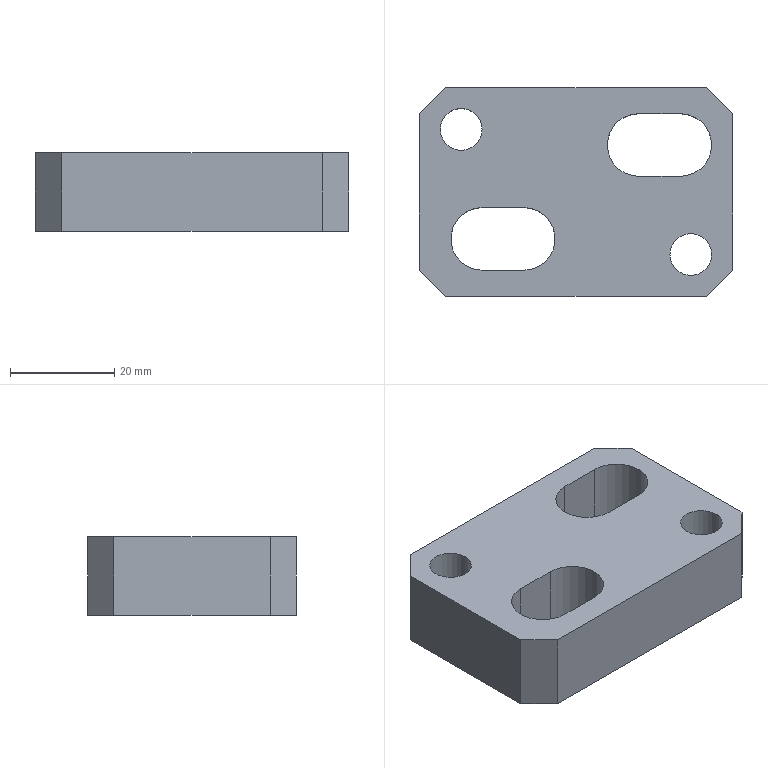Part | NX | features solid 2 | 1 solid | 20 faces | box 60 x 40 x 15 mm | volume 27469 mm3 | plane 14 | cylinder 6 | commonest cylinder face diameters 12 x4 8 x2
STEP:
#1=CARTESIAN_POINT('',(-940.,-92.5,-50.));
#2=VERTEX_POINT('',#1);
#3=CARTESIAN_POINT('',(-890.,-92.5,-50.));
#4=VERTEX_POINT('',#3);
#5=CARTESIAN_POINT('',(-945.,-92.5,-50.));
#6=DIRECTION('',(1.,0.,0.));
#7=VECTOR('',#6,1000.);
#8=LINE('',#5,#7);
#9=EDGE_CURVE('',#2,#4,#8,.T.);
#10=ORIENTED_EDGE('',*,*,#9,.T.);
#11=CARTESIAN_POINT('',(-890.,-92.5,-35.));
#12=VERTEX_POINT('',#11);
#13=CARTESIAN_POINT('',(-890.,-92.5,-35.));
#14=DIRECTION('',(0.,0.,-1.));
#15=VECTOR('',#14,1000.);
#16=LINE('',#13,#15);
#17=EDGE_CURVE('',#12,#4,#16,.T.);
#18=ORIENTED_EDGE('',*,*,#17,.F.);
#19=CARTESIAN_POINT('',(-940.,-92.5,-35.));
#20=VERTEX_POINT('',#19);
#21=CARTESIAN_POINT('',(-945.,-92.5,-35.));
#22=DIRECTION('',(1.,0.,0.));
#23=VECTOR('',#22,1000.);
#24=LINE('',#21,#23);
#25=EDGE_CURVE('',#20,#12,#24,.T.);
#26=ORIENTED_EDGE('',*,*,#25,.F.);
#27=CARTESIAN_POINT('',(-940.,-92.5,-35.));
#28=DIRECTION('',(0.,0.,-1.));
#29=VECTOR('',#28,1000.);
#30=LINE('',#27,#29);
#31=EDGE_CURVE('',#20,#2,#30,.T.);
#32=ORIENTED_EDGE('',*,*,#31,.T.);
#33=EDGE_LOOP('',(#10,#18,#26,#32));
#34=FACE_BOUND('',#33,.T.);
#35=CARTESIAN_POINT('',(-945.,-92.5,-35.));
#36=DIRECTION('',(0.,-1.,0.));
#37=DIRECTION('',(0.,0.,-1.));
#38=AXIS2_PLACEMENT_3D('',#35,#36,#37);
#39=PLANE('',#38);
#40=ADVANCED_FACE('',(#34),#39,.T.);
#41=CARTESIAN_POINT('',(-885.,-87.5,-50.));
#42=VERTEX_POINT('',#41);
#43=CARTESIAN_POINT('',(-890.,-92.5,-50.));
#44=DIRECTION('',(0.7071,0.7071,0.));
#45=VECTOR('',#44,1000.);
#46=LINE('',#43,#45);
#47=EDGE_CURVE('',#4,#42,#46,.T.);
#48=ORIENTED_EDGE('',*,*,#47,.T.);
#49=CARTESIAN_POINT('',(-885.,-87.5,-35.));
#50=VERTEX_POINT('',#49);
#51=CARTESIAN_POINT('',(-885.,-87.5,-35.));
#52=DIRECTION('',(0.,0.,-1.));
#53=VECTOR('',#52,1000.);
#54=LINE('',#51,#53);
#55=EDGE_CURVE('',#50,#42,#54,.T.);
#56=ORIENTED_EDGE('',*,*,#55,.F.);
#57=CARTESIAN_POINT('',(-890.,-92.5,-35.));
#58=DIRECTION('',(0.7071,0.7071,0.));
#59=VECTOR('',#58,1000.);
#60=LINE('',#57,#59);
#61=EDGE_CURVE('',#12,#50,#60,.T.);
#62=ORIENTED_EDGE('',*,*,#61,.F.);
#63=ORIENTED_EDGE('',*,*,#17,.T.);
#64=EDGE_LOOP('',(#48,#56,#62,#63));
#65=FACE_BOUND('',#64,.T.);
#66=CARTESIAN_POINT('',(-890.,-92.5,-35.));
#67=DIRECTION('',(0.7071,-0.7071,0.));
#68=DIRECTION('',(-0.7071,-0.7071,0.));
#69=AXIS2_PLACEMENT_3D('',#66,#67,#68);
#70=PLANE('',#69);
#71=ADVANCED_FACE('',(#65),#70,.T.);
#72=CARTESIAN_POINT('',(-885.,-57.5,-50.));
#73=VERTEX_POINT('',#72);
#74=CARTESIAN_POINT('',(-885.,-87.5,-50.));
#75=DIRECTION('',(0.,1.,0.));
#76=VECTOR('',#75,1000.);
#77=LINE('',#74,#76);
#78=EDGE_CURVE('',#42,#73,#77,.T.);
#79=ORIENTED_EDGE('',*,*,#78,.T.);
#80=CARTESIAN_POINT('',(-885.,-57.5,-35.));
#81=VERTEX_POINT('',#80);
#82=CARTESIAN_POINT('',(-885.,-57.5,-35.));
#83=DIRECTION('',(0.,0.,-1.));
#84=VECTOR('',#83,1000.);
#85=LINE('',#82,#84);
#86=EDGE_CURVE('',#81,#73,#85,.T.);
#87=ORIENTED_EDGE('',*,*,#86,.F.);
#88=CARTESIAN_POINT('',(-885.,-87.5,-35.));
#89=DIRECTION('',(0.,1.,0.));
#90=VECTOR('',#89,1000.);
#91=LINE('',#88,#90);
#92=EDGE_CURVE('',#50,#81,#91,.T.);
#93=ORIENTED_EDGE('',*,*,#92,.F.);
#94=ORIENTED_EDGE('',*,*,#55,.T.);
#95=EDGE_LOOP('',(#79,#87,#93,#94));
#96=FACE_BOUND('',#95,.T.);
#97=CARTESIAN_POINT('',(-885.,-87.5,-35.));
#98=DIRECTION('',(1.,0.,0.));
#99=DIRECTION('',(0.,-1.,0.));
#100=AXIS2_PLACEMENT_3D('',#97,#98,#99);
#101=PLANE('',#100);
#102=ADVANCED_FACE('',(#96),#101,.T.);
#103=CARTESIAN_POINT('',(-890.,-52.5,-50.));
#104=VERTEX_POINT('',#103);
#105=CARTESIAN_POINT('',(-885.,-57.5,-50.));
#106=DIRECTION('',(-0.7071,0.7071,0.));
#107=VECTOR('',#106,1000.);
#108=LINE('',#105,#107);
#109=EDGE_CURVE('',#73,#104,#108,.T.);
#110=ORIENTED_EDGE('',*,*,#109,.T.);
#111=CARTESIAN_POINT('',(-890.,-52.5,-35.));
#112=VERTEX_POINT('',#111);
#113=CARTESIAN_POINT('',(-890.,-52.5,-35.));
#114=DIRECTION('',(0.,0.,-1.));
#115=VECTOR('',#114,1000.);
#116=LINE('',#113,#115);
#117=EDGE_CURVE('',#112,#104,#116,.T.);
#118=ORIENTED_EDGE('',*,*,#117,.F.);
#119=CARTESIAN_POINT('',(-885.,-57.5,-35.));
#120=DIRECTION('',(-0.7071,0.7071,0.));
#121=VECTOR('',#120,1000.);
#122=LINE('',#119,#121);
#123=EDGE_CURVE('',#81,#112,#122,.T.);
#124=ORIENTED_EDGE('',*,*,#123,.F.);
#125=ORIENTED_EDGE('',*,*,#86,.T.);
#126=EDGE_LOOP('',(#110,#118,#124,#125));
#127=FACE_BOUND('',#126,.T.);
#128=CARTESIAN_POINT('',(-885.,-57.5,-35.));
#129=DIRECTION('',(0.7071,0.7071,0.));
#130=DIRECTION('',(0.7071,-0.7071,0.));
#131=AXIS2_PLACEMENT_3D('',#128,#129,#130);
#132=PLANE('',#131);
#133=ADVANCED_FACE('',(#127),#132,.T.);
#134=CARTESIAN_POINT('',(-940.,-52.5,-35.));
#135=VERTEX_POINT('',#134);
#136=CARTESIAN_POINT('',(-915.,-52.5,-35.));
#137=DIRECTION('',(-1.,0.,0.));
#138=VECTOR('',#137,1000.);
#139=LINE('',#136,#138);
#140=EDGE_CURVE('',#112,#135,#139,.T.);
#141=ORIENTED_EDGE('',*,*,#140,.F.);
#142=ORIENTED_EDGE('',*,*,#117,.T.);
#143=CARTESIAN_POINT('',(-940.,-52.5,-50.));
#144=VERTEX_POINT('',#143);
#145=CARTESIAN_POINT('',(-915.,-52.5,-50.));
#146=DIRECTION('',(-1.,0.,0.));
#147=VECTOR('',#146,1000.);
#148=LINE('',#145,#147);
#149=EDGE_CURVE('',#104,#144,#148,.T.);
#150=ORIENTED_EDGE('',*,*,#149,.T.);
#151=CARTESIAN_POINT('',(-940.,-52.5,-35.));
#152=DIRECTION('',(0.,0.,-1.));
#153=VECTOR('',#152,1000.);
#154=LINE('',#151,#153);
#155=EDGE_CURVE('',#135,#144,#154,.T.);
#156=ORIENTED_EDGE('',*,*,#155,.F.);
#157=EDGE_LOOP('',(#141,#142,#150,#156));
#158=FACE_BOUND('',#157,.T.);
#159=CARTESIAN_POINT('',(-915.,-52.5,-35.));
#160=DIRECTION('',(0.,1.,0.));
#161=DIRECTION('',(1.,0.,0.));
#162=AXIS2_PLACEMENT_3D('',#159,#160,#161);
#163=PLANE('',#162);
#164=ADVANCED_FACE('',(#158),#163,.T.);
#165=CARTESIAN_POINT('',(-903.,-69.5,-50.));
#166=VERTEX_POINT('',#165);
#167=CARTESIAN_POINT('',(-903.,-57.5,-50.));
#168=VERTEX_POINT('',#167);
#169=CARTESIAN_POINT('',(-903.,-63.5,-50.));
#170=DIRECTION('',(0.,0.,-1.));
#171=DIRECTION('',(-1.,0.,0.));
#172=AXIS2_PLACEMENT_3D('',#169,#170,#171);
#173=CIRCLE('',#172,6.);
#174=EDGE_CURVE('',#166,#168,#173,.T.);
#175=ORIENTED_EDGE('',*,*,#174,.T.);
#176=CARTESIAN_POINT('',(-903.,-57.5,-35.));
#177=VERTEX_POINT('',#176);
#178=CARTESIAN_POINT('',(-903.,-57.5,-35.));
#179=DIRECTION('',(0.,0.,-1.));
#180=VECTOR('',#179,1000.);
#181=LINE('',#178,#180);
#182=EDGE_CURVE('',#177,#168,#181,.T.);
#183=ORIENTED_EDGE('',*,*,#182,.F.);
#184=CARTESIAN_POINT('',(-903.,-69.5,-35.));
#185=VERTEX_POINT('',#184);
#186=CARTESIAN_POINT('',(-903.,-63.5,-35.));
#187=DIRECTION('',(0.,0.,-1.));
#188=DIRECTION('',(-1.,0.,0.));
#189=AXIS2_PLACEMENT_3D('',#186,#187,#188);
#190=CIRCLE('',#189,6.);
#191=EDGE_CURVE('',#185,#177,#190,.T.);
#192=ORIENTED_EDGE('',*,*,#191,.F.);
#193=CARTESIAN_POINT('',(-903.,-69.5,-35.));
#194=DIRECTION('',(0.,0.,-1.));
#195=VECTOR('',#194,1000.);
#196=LINE('',#193,#195);
#197=EDGE_CURVE('',#185,#166,#196,.T.);
#198=ORIENTED_EDGE('',*,*,#197,.T.);
#199=EDGE_LOOP('',(#175,#183,#192,#198));
#200=FACE_BOUND('',#199,.T.);
#201=CARTESIAN_POINT('',(-903.,-63.5,-35.));
#202=DIRECTION('',(0.,0.,-1.));
#203=DIRECTION('',(1.,0.,0.));
#204=AXIS2_PLACEMENT_3D('',#201,#202,#203);
#205=CYLINDRICAL_SURFACE('',#204,6.);
#206=ADVANCED_FACE('',(#200),#205,.F.);
#207=CARTESIAN_POINT('',(-895.,-57.5,-50.));
#208=VERTEX_POINT('',#207);
#209=CARTESIAN_POINT('',(-895.,-57.5,-50.));
#210=DIRECTION('',(-1.,0.,0.));
#211=VECTOR('',#210,1000.);
#212=LINE('',#209,#211);
#213=EDGE_CURVE('',#208,#168,#212,.T.);
#214=ORIENTED_EDGE('',*,*,#213,.F.);
#215=CARTESIAN_POINT('',(-895.,-57.5,-35.));
#216=VERTEX_POINT('',#215);
#217=CARTESIAN_POINT('',(-895.,-57.5,-35.));
#218=DIRECTION('',(0.,0.,-1.));
#219=VECTOR('',#218,1000.);
#220=LINE('',#217,#219);
#221=EDGE_CURVE('',#216,#208,#220,.T.);
#222=ORIENTED_EDGE('',*,*,#221,.F.);
#223=CARTESIAN_POINT('',(-895.,-57.5,-35.));
#224=DIRECTION('',(-1.,0.,0.));
#225=VECTOR('',#224,1000.);
#226=LINE('',#223,#225);
#227=EDGE_CURVE('',#216,#177,#226,.T.);
#228=ORIENTED_EDGE('',*,*,#227,.T.);
#229=ORIENTED_EDGE('',*,*,#182,.T.);
#230=EDGE_LOOP('',(#214,#222,#228,#229));
#231=FACE_BOUND('',#230,.T.);
#232=CARTESIAN_POINT('',(-895.,-57.5,-35.));
#233=DIRECTION('',(0.,1.,0.));
#234=DIRECTION('',(0.,0.,1.));
#235=AXIS2_PLACEMENT_3D('',#232,#233,#234);
#236=PLANE('',#235);
#237=ADVANCED_FACE('',(#231),#236,.F.);
#238=CARTESIAN_POINT('',(-895.,-69.5,-50.));
#239=VERTEX_POINT('',#238);
#240=CARTESIAN_POINT('',(-895.,-63.5,-50.));
#241=DIRECTION('',(0.,0.,-1.));
#242=DIRECTION('',(-1.,0.,0.));
#243=AXIS2_PLACEMENT_3D('',#240,#241,#242);
#244=CIRCLE('',#243,6.);
#245=EDGE_CURVE('',#208,#239,#244,.T.);
#246=ORIENTED_EDGE('',*,*,#245,.T.);
#247=CARTESIAN_POINT('',(-895.,-69.5,-35.));
#248=VERTEX_POINT('',#247);
#249=CARTESIAN_POINT('',(-895.,-69.5,-35.));
#250=DIRECTION('',(0.,0.,-1.));
#251=VECTOR('',#250,1000.);
#252=LINE('',#249,#251);
#253=EDGE_CURVE('',#248,#239,#252,.T.);
#254=ORIENTED_EDGE('',*,*,#253,.F.);
#255=CARTESIAN_POINT('',(-895.,-63.5,-35.));
#256=DIRECTION('',(0.,0.,-1.));
#257=DIRECTION('',(-1.,0.,0.));
#258=AXIS2_PLACEMENT_3D('',#255,#256,#257);
#259=CIRCLE('',#258,6.);
#260=EDGE_CURVE('',#216,#248,#259,.T.);
#261=ORIENTED_EDGE('',*,*,#260,.F.);
#262=ORIENTED_EDGE('',*,*,#221,.T.);
#263=EDGE_LOOP('',(#246,#254,#261,#262));
#264=FACE_BOUND('',#263,.T.);
#265=CARTESIAN_POINT('',(-895.,-63.5,-35.));
#266=DIRECTION('',(0.,0.,-1.));
#267=DIRECTION('',(1.,0.,0.));
#268=AXIS2_PLACEMENT_3D('',#265,#266,#267);
#269=CYLINDRICAL_SURFACE('',#268,6.);
#270=ADVANCED_FACE('',(#264),#269,.F.);
#271=CARTESIAN_POINT('',(-903.,-69.5,-35.));
#272=DIRECTION('',(1.,0.,0.));
#273=VECTOR('',#272,1000.);
#274=LINE('',#271,#273);
#275=EDGE_CURVE('',#185,#248,#274,.T.);
#276=ORIENTED_EDGE('',*,*,#275,.T.);
#277=ORIENTED_EDGE('',*,*,#253,.T.);
#278=CARTESIAN_POINT('',(-903.,-69.5,-50.));
#279=DIRECTION('',(1.,0.,0.));
#280=VECTOR('',#279,1000.);
#281=LINE('',#278,#280);
#282=EDGE_CURVE('',#166,#239,#281,.T.);
#283=ORIENTED_EDGE('',*,*,#282,.F.);
#284=ORIENTED_EDGE('',*,*,#197,.F.);
#285=EDGE_LOOP('',(#276,#277,#283,#284));
#286=FACE_BOUND('',#285,.T.);
#287=CARTESIAN_POINT('',(-903.,-69.5,-35.));
#288=DIRECTION('',(0.,-1.,0.));
#289=DIRECTION('',(-1.,0.,0.));
#290=AXIS2_PLACEMENT_3D('',#287,#288,#289);
#291=PLANE('',#290);
#292=ADVANCED_FACE('',(#286),#291,.F.);
#293=CARTESIAN_POINT('',(-941.,-60.5,-35.));
#294=VERTEX_POINT('',#293);
#295=CARTESIAN_POINT('',(-937.,-60.5,-35.));
#296=DIRECTION('',(0.,0.,-1.));
#297=DIRECTION('',(-1.,0.,0.));
#298=AXIS2_PLACEMENT_3D('',#295,#296,#297);
#299=CIRCLE('',#298,4.);
#300=EDGE_CURVE('',#294,#294,#299,.T.);
#301=ORIENTED_EDGE('',*,*,#300,.F.);
#302=EDGE_LOOP('',(#301));
#303=FACE_BOUND('',#302,.T.);
#304=CARTESIAN_POINT('',(-941.,-60.5,-50.));
#305=VERTEX_POINT('',#304);
#306=CARTESIAN_POINT('',(-937.,-60.5,-50.));
#307=DIRECTION('',(0.,0.,-1.));
#308=DIRECTION('',(-1.,0.,0.));
#309=AXIS2_PLACEMENT_3D('',#306,#307,#308);
#310=CIRCLE('',#309,4.);
#311=EDGE_CURVE('',#305,#305,#310,.T.);
#312=ORIENTED_EDGE('',*,*,#311,.T.);
#313=EDGE_LOOP('',(#312));
#314=FACE_BOUND('',#313,.T.);
#315=CARTESIAN_POINT('',(-937.,-60.5,-35.));
#316=DIRECTION('',(0.,0.,-1.));
#317=DIRECTION('',(1.,0.,0.));
#318=AXIS2_PLACEMENT_3D('',#315,#316,#317);
#319=CYLINDRICAL_SURFACE('',#318,4.);
#320=ADVANCED_FACE('',(#303,#314),#319,.F.);
#321=CARTESIAN_POINT('',(-933.,-87.5,-50.));
#322=VERTEX_POINT('',#321);
#323=CARTESIAN_POINT('',(-933.,-75.5,-50.));
#324=VERTEX_POINT('',#323);
#325=CARTESIAN_POINT('',(-933.,-81.5,-50.));
#326=DIRECTION('',(0.,0.,-1.));
#327=DIRECTION('',(-1.,0.,0.));
#328=AXIS2_PLACEMENT_3D('',#325,#326,#327);
#329=CIRCLE('',#328,6.);
#330=EDGE_CURVE('',#322,#324,#329,.T.);
#331=ORIENTED_EDGE('',*,*,#330,.T.);
#332=CARTESIAN_POINT('',(-933.,-75.5,-35.));
#333=VERTEX_POINT('',#332);
#334=CARTESIAN_POINT('',(-933.,-75.5,-35.));
#335=DIRECTION('',(0.,0.,-1.));
#336=VECTOR('',#335,1000.);
#337=LINE('',#334,#336);
#338=EDGE_CURVE('',#333,#324,#337,.T.);
#339=ORIENTED_EDGE('',*,*,#338,.F.);
#340=CARTESIAN_POINT('',(-933.,-87.5,-35.));
#341=VERTEX_POINT('',#340);
#342=CARTESIAN_POINT('',(-933.,-81.5,-35.));
#343=DIRECTION('',(0.,0.,-1.));
#344=DIRECTION('',(-1.,0.,0.));
#345=AXIS2_PLACEMENT_3D('',#342,#343,#344);
#346=CIRCLE('',#345,6.);
#347=EDGE_CURVE('',#341,#333,#346,.T.);
#348=ORIENTED_EDGE('',*,*,#347,.F.);
#349=CARTESIAN_POINT('',(-933.,-87.5,-35.));
#350=DIRECTION('',(0.,0.,-1.));
#351=VECTOR('',#350,1000.);
#352=LINE('',#349,#351);
#353=EDGE_CURVE('',#341,#322,#352,.T.);
#354=ORIENTED_EDGE('',*,*,#353,.T.);
#355=EDGE_LOOP('',(#331,#339,#348,#354));
#356=FACE_BOUND('',#355,.T.);
#357=CARTESIAN_POINT('',(-933.,-81.5,-35.));
#358=DIRECTION('',(0.,0.,-1.));
#359=DIRECTION('',(1.,0.,0.));
#360=AXIS2_PLACEMENT_3D('',#357,#358,#359);
#361=CYLINDRICAL_SURFACE('',#360,6.);
#362=ADVANCED_FACE('',(#356),#361,.F.);
#363=CARTESIAN_POINT('',(-925.,-75.5,-50.));
#364=VERTEX_POINT('',#363);
#365=CARTESIAN_POINT('',(-925.,-75.5,-50.));
#366=DIRECTION('',(-1.,0.,0.));
#367=VECTOR('',#366,1000.);
#368=LINE('',#365,#367);
#369=EDGE_CURVE('',#364,#324,#368,.T.);
#370=ORIENTED_EDGE('',*,*,#369,.F.);
#371=CARTESIAN_POINT('',(-925.,-75.5,-35.));
#372=VERTEX_POINT('',#371);
#373=CARTESIAN_POINT('',(-925.,-75.5,-35.));
#374=DIRECTION('',(0.,0.,-1.));
#375=VECTOR('',#374,1000.);
#376=LINE('',#373,#375);
#377=EDGE_CURVE('',#372,#364,#376,.T.);
#378=ORIENTED_EDGE('',*,*,#377,.F.);
#379=CARTESIAN_POINT('',(-925.,-75.5,-35.));
#380=DIRECTION('',(-1.,0.,0.));
#381=VECTOR('',#380,1000.);
#382=LINE('',#379,#381);
#383=EDGE_CURVE('',#372,#333,#382,.T.);
#384=ORIENTED_EDGE('',*,*,#383,.T.);
#385=ORIENTED_EDGE('',*,*,#338,.T.);
#386=EDGE_LOOP('',(#370,#378,#384,#385));
#387=FACE_BOUND('',#386,.T.);
#388=CARTESIAN_POINT('',(-925.,-75.5,-35.));
#389=DIRECTION('',(0.,1.,0.));
#390=DIRECTION('',(1.,0.,0.));
#391=AXIS2_PLACEMENT_3D('',#388,#389,#390);
#392=PLANE('',#391);
#393=ADVANCED_FACE('',(#387),#392,.F.);
#394=CARTESIAN_POINT('',(-925.,-87.5,-35.));
#395=VERTEX_POINT('',#394);
#396=CARTESIAN_POINT('',(-925.,-81.5,-35.));
#397=DIRECTION('',(0.,0.,-1.));
#398=DIRECTION('',(-1.,0.,0.));
#399=AXIS2_PLACEMENT_3D('',#396,#397,#398);
#400=CIRCLE('',#399,6.);
#401=EDGE_CURVE('',#372,#395,#400,.T.);
#402=ORIENTED_EDGE('',*,*,#401,.F.);
#403=ORIENTED_EDGE('',*,*,#377,.T.);
#404=CARTESIAN_POINT('',(-925.,-87.5,-50.));
#405=VERTEX_POINT('',#404);
#406=CARTESIAN_POINT('',(-925.,-81.5,-50.));
#407=DIRECTION('',(0.,0.,-1.));
#408=DIRECTION('',(-1.,0.,0.));
#409=AXIS2_PLACEMENT_3D('',#406,#407,#408);
#410=CIRCLE('',#409,6.);
#411=EDGE_CURVE('',#364,#405,#410,.T.);
#412=ORIENTED_EDGE('',*,*,#411,.T.);
#413=CARTESIAN_POINT('',(-925.,-87.5,-35.));
#414=DIRECTION('',(0.,0.,-1.));
#415=VECTOR('',#414,1000.);
#416=LINE('',#413,#415);
#417=EDGE_CURVE('',#395,#405,#416,.T.);
#418=ORIENTED_EDGE('',*,*,#417,.F.);
#419=EDGE_LOOP('',(#402,#403,#412,#418));
#420=FACE_BOUND('',#419,.T.);
#421=CARTESIAN_POINT('',(-925.,-81.5,-35.));
#422=DIRECTION('',(0.,0.,-1.));
#423=DIRECTION('',(1.,0.,0.));
#424=AXIS2_PLACEMENT_3D('',#421,#422,#423);
#425=CYLINDRICAL_SURFACE('',#424,6.);
#426=ADVANCED_FACE('',(#420),#425,.F.);
#427=CARTESIAN_POINT('',(-933.,-87.5,-50.));
#428=DIRECTION('',(1.,0.,0.));
#429=VECTOR('',#428,1000.);
#430=LINE('',#427,#429);
#431=EDGE_CURVE('',#322,#405,#430,.T.);
#432=ORIENTED_EDGE('',*,*,#431,.F.);
#433=ORIENTED_EDGE('',*,*,#353,.F.);
#434=CARTESIAN_POINT('',(-933.,-87.5,-35.));
#435=DIRECTION('',(1.,0.,0.));
#436=VECTOR('',#435,1000.);
#437=LINE('',#434,#436);
#438=EDGE_CURVE('',#341,#395,#437,.T.);
#439=ORIENTED_EDGE('',*,*,#438,.T.);
#440=ORIENTED_EDGE('',*,*,#417,.T.);
#441=EDGE_LOOP('',(#432,#433,#439,#440));
#442=FACE_BOUND('',#441,.T.);
#443=CARTESIAN_POINT('',(-933.,-87.5,-35.));
#444=DIRECTION('',(0.,-1.,0.));
#445=DIRECTION('',(0.,0.,-1.));
#446=AXIS2_PLACEMENT_3D('',#443,#444,#445);
#447=PLANE('',#446);
#448=ADVANCED_FACE('',(#442),#447,.F.);
#449=CARTESIAN_POINT('',(-897.,-84.5,-35.));
#450=VERTEX_POINT('',#449);
#451=CARTESIAN_POINT('',(-893.,-84.5,-35.));
#452=DIRECTION('',(0.,0.,-1.));
#453=DIRECTION('',(-1.,0.,0.));
#454=AXIS2_PLACEMENT_3D('',#451,#452,#453);
#455=CIRCLE('',#454,4.);
#456=EDGE_CURVE('',#450,#450,#455,.T.);
#457=ORIENTED_EDGE('',*,*,#456,.F.);
#458=EDGE_LOOP('',(#457));
#459=FACE_BOUND('',#458,.T.);
#460=CARTESIAN_POINT('',(-897.,-84.5,-50.));
#461=VERTEX_POINT('',#460);
#462=CARTESIAN_POINT('',(-893.,-84.5,-50.));
#463=DIRECTION('',(0.,0.,-1.));
#464=DIRECTION('',(-1.,0.,0.));
#465=AXIS2_PLACEMENT_3D('',#462,#463,#464);
#466=CIRCLE('',#465,4.);
#467=EDGE_CURVE('',#461,#461,#466,.T.);
#468=ORIENTED_EDGE('',*,*,#467,.T.);
#469=EDGE_LOOP('',(#468));
#470=FACE_BOUND('',#469,.T.);
#471=CARTESIAN_POINT('',(-893.,-84.5,-35.));
#472=DIRECTION('',(0.,0.,-1.));
#473=DIRECTION('',(1.,0.,0.));
#474=AXIS2_PLACEMENT_3D('',#471,#472,#473);
#475=CYLINDRICAL_SURFACE('',#474,4.);
#476=ADVANCED_FACE('',(#459,#470),#475,.F.);
#477=CARTESIAN_POINT('',(-945.,-57.5,-50.));
#478=VERTEX_POINT('',#477);
#479=CARTESIAN_POINT('',(-940.,-52.5,-50.));
#480=DIRECTION('',(-0.7071,-0.7071,0.));
#481=VECTOR('',#480,1000.);
#482=LINE('',#479,#481);
#483=EDGE_CURVE('',#144,#478,#482,.T.);
#484=ORIENTED_EDGE('',*,*,#483,.T.);
#485=CARTESIAN_POINT('',(-945.,-57.5,-35.));
#486=VERTEX_POINT('',#485);
#487=CARTESIAN_POINT('',(-945.,-57.5,-35.));
#488=DIRECTION('',(0.,0.,-1.));
#489=VECTOR('',#488,1000.);
#490=LINE('',#487,#489);
#491=EDGE_CURVE('',#486,#478,#490,.T.);
#492=ORIENTED_EDGE('',*,*,#491,.F.);
#493=CARTESIAN_POINT('',(-940.,-52.5,-35.));
#494=DIRECTION('',(-0.7071,-0.7071,0.));
#495=VECTOR('',#494,1000.);
#496=LINE('',#493,#495);
#497=EDGE_CURVE('',#135,#486,#496,.T.);
#498=ORIENTED_EDGE('',*,*,#497,.F.);
#499=ORIENTED_EDGE('',*,*,#155,.T.);
#500=EDGE_LOOP('',(#484,#492,#498,#499));
#501=FACE_BOUND('',#500,.T.);
#502=CARTESIAN_POINT('',(-940.,-52.5,-35.));
#503=DIRECTION('',(-0.7071,0.7071,0.));
#504=DIRECTION('',(0.7071,0.7071,0.));
#505=AXIS2_PLACEMENT_3D('',#502,#503,#504);
#506=PLANE('',#505);
#507=ADVANCED_FACE('',(#501),#506,.T.);
#508=CARTESIAN_POINT('',(-945.,-87.5,-50.));
#509=VERTEX_POINT('',#508);
#510=CARTESIAN_POINT('',(-945.,-87.5,-50.));
#511=DIRECTION('',(0.7071,-0.7071,0.));
#512=VECTOR('',#511,1000.);
#513=LINE('',#510,#512);
#514=EDGE_CURVE('',#509,#2,#513,.T.);
#515=ORIENTED_EDGE('',*,*,#514,.T.);
#516=ORIENTED_EDGE('',*,*,#31,.F.);
#517=CARTESIAN_POINT('',(-945.,-87.5,-35.));
#518=VERTEX_POINT('',#517);
#519=CARTESIAN_POINT('',(-945.,-87.5,-35.));
#520=DIRECTION('',(0.7071,-0.7071,0.));
#521=VECTOR('',#520,1000.);
#522=LINE('',#519,#521);
#523=EDGE_CURVE('',#518,#20,#522,.T.);
#524=ORIENTED_EDGE('',*,*,#523,.F.);
#525=CARTESIAN_POINT('',(-945.,-87.5,-35.));
#526=DIRECTION('',(0.,0.,-1.));
#527=VECTOR('',#526,1000.);
#528=LINE('',#525,#527);
#529=EDGE_CURVE('',#518,#509,#528,.T.);
#530=ORIENTED_EDGE('',*,*,#529,.T.);
#531=EDGE_LOOP('',(#515,#516,#524,#530));
#532=FACE_BOUND('',#531,.T.);
#533=CARTESIAN_POINT('',(-945.,-87.5,-35.));
#534=DIRECTION('',(-0.7071,-0.7071,0.));
#535=DIRECTION('',(-0.7071,0.7071,0.));
#536=AXIS2_PLACEMENT_3D('',#533,#534,#535);
#537=PLANE('',#536);
#538=ADVANCED_FACE('',(#532),#537,.T.);
#539=CARTESIAN_POINT('',(-945.,-72.5,-35.));
#540=DIRECTION('',(0.,1.,0.));
#541=VECTOR('',#540,1000.);
#542=LINE('',#539,#541);
#543=EDGE_CURVE('',#518,#486,#542,.T.);
#544=ORIENTED_EDGE('',*,*,#543,.T.);
#545=ORIENTED_EDGE('',*,*,#491,.T.);
#546=CARTESIAN_POINT('',(-945.,-45.5,-50.));
#547=DIRECTION('',(0.,-1.,0.));
#548=VECTOR('',#547,1000.);
#549=LINE('',#546,#548);
#550=EDGE_CURVE('',#478,#509,#549,.T.);
#551=ORIENTED_EDGE('',*,*,#550,.T.);
#552=ORIENTED_EDGE('',*,*,#529,.F.);
#553=EDGE_LOOP('',(#544,#545,#551,#552));
#554=FACE_BOUND('',#553,.T.);
#555=CARTESIAN_POINT('',(-945.,-87.5,-35.));
#556=DIRECTION('',(-1.,0.,0.));
#557=DIRECTION('',(0.,-1.,0.));
#558=AXIS2_PLACEMENT_3D('',#555,#556,#557);
#559=PLANE('',#558);
#560=ADVANCED_FACE('',(#554),#559,.T.);
#561=ORIENTED_EDGE('',*,*,#467,.F.);
#562=EDGE_LOOP('',(#561));
#563=FACE_BOUND('',#562,.T.);
#564=ORIENTED_EDGE('',*,*,#431,.T.);
#565=ORIENTED_EDGE('',*,*,#411,.F.);
#566=ORIENTED_EDGE('',*,*,#369,.T.);
#567=ORIENTED_EDGE('',*,*,#330,.F.);
#568=EDGE_LOOP('',(#564,#565,#566,#567));
#569=FACE_BOUND('',#568,.T.);
#570=ORIENTED_EDGE('',*,*,#311,.F.);
#571=EDGE_LOOP('',(#570));
#572=FACE_BOUND('',#571,.T.);
#573=ORIENTED_EDGE('',*,*,#282,.T.);
#574=ORIENTED_EDGE('',*,*,#245,.F.);
#575=ORIENTED_EDGE('',*,*,#213,.T.);
#576=ORIENTED_EDGE('',*,*,#174,.F.);
#577=EDGE_LOOP('',(#573,#574,#575,#576));
#578=FACE_BOUND('',#577,.T.);
#579=ORIENTED_EDGE('',*,*,#514,.F.);
#580=ORIENTED_EDGE('',*,*,#550,.F.);
#581=ORIENTED_EDGE('',*,*,#483,.F.);
#582=ORIENTED_EDGE('',*,*,#149,.F.);
#583=ORIENTED_EDGE('',*,*,#109,.F.);
#584=ORIENTED_EDGE('',*,*,#78,.F.);
#585=ORIENTED_EDGE('',*,*,#47,.F.);
#586=ORIENTED_EDGE('',*,*,#9,.F.);
#587=EDGE_LOOP('',(#579,#580,#581,#582,#583,#584,#585,#586));
#588=FACE_BOUND('',#587,.T.);
#589=CARTESIAN_POINT('',(-977.,-45.5,-50.));
#590=DIRECTION('',(0.,0.,1.));
#591=DIRECTION('',(0.,-1.,0.));
#592=AXIS2_PLACEMENT_3D('',#589,#590,#591);
#593=PLANE('',#592);
#594=ADVANCED_FACE('',(#563,#569,#572,#578,#588),#593,.F.);
#595=ORIENTED_EDGE('',*,*,#497,.T.);
#596=ORIENTED_EDGE('',*,*,#543,.F.);
#597=ORIENTED_EDGE('',*,*,#523,.T.);
#598=ORIENTED_EDGE('',*,*,#25,.T.);
#599=ORIENTED_EDGE('',*,*,#61,.T.);
#600=ORIENTED_EDGE('',*,*,#92,.T.);
#601=ORIENTED_EDGE('',*,*,#123,.T.);
#602=ORIENTED_EDGE('',*,*,#140,.T.);
#603=EDGE_LOOP('',(#595,#596,#597,#598,#599,#600,#601,#602));
#604=FACE_BOUND('',#603,.T.);
#605=ORIENTED_EDGE('',*,*,#456,.T.);
#606=EDGE_LOOP('',(#605));
#607=FACE_BOUND('',#606,.T.);
#608=ORIENTED_EDGE('',*,*,#347,.T.);
#609=ORIENTED_EDGE('',*,*,#383,.F.);
#610=ORIENTED_EDGE('',*,*,#401,.T.);
#611=ORIENTED_EDGE('',*,*,#438,.F.);
#612=EDGE_LOOP('',(#608,#609,#610,#611));
#613=FACE_BOUND('',#612,.T.);
#614=ORIENTED_EDGE('',*,*,#300,.T.);
#615=EDGE_LOOP('',(#614));
#616=FACE_BOUND('',#615,.T.);
#617=ORIENTED_EDGE('',*,*,#260,.T.);
#618=ORIENTED_EDGE('',*,*,#275,.F.);
#619=ORIENTED_EDGE('',*,*,#191,.T.);
#620=ORIENTED_EDGE('',*,*,#227,.F.);
#621=EDGE_LOOP('',(#617,#618,#619,#620));
#622=FACE_BOUND('',#621,.T.);
#623=CARTESIAN_POINT('',(-977.,-45.5,-35.));
#624=DIRECTION('',(0.,0.,1.));
#625=DIRECTION('',(0.,-1.,0.));
#626=AXIS2_PLACEMENT_3D('',#623,#624,#625);
#627=PLANE('',#626);
#628=ADVANCED_FACE('',(#604,#607,#613,#616,#622),#627,.T.);
#629=CLOSED_SHELL('',(#40,#71,#102,#133,#164,#206,#237,#270,#292,#320,#362,#393,#426,#448,#476,#507,#538,#560,#594,#628));
#630=MANIFOLD_SOLID_BREP('',#629);
#631=(LENGTH_UNIT()NAMED_UNIT(*)SI_UNIT(.MILLI.,.METRE.));
#632=UNCERTAINTY_MEASURE_WITH_UNIT(LENGTH_MEASURE(0.00001),#631,'','');
#633=(NAMED_UNIT(*)PLANE_ANGLE_UNIT()SI_UNIT($,.RADIAN.));
#634=(NAMED_UNIT(*)SI_UNIT($,.STERADIAN.)SOLID_ANGLE_UNIT());
#635=(GEOMETRIC_REPRESENTATION_CONTEXT(3)GLOBAL_UNCERTAINTY_ASSIGNED_CONTEXT((#632))GLOBAL_UNIT_ASSIGNED_CONTEXT((#631,#633,#634))REPRESENTATION_CONTEXT('',''));
#636=ADVANCED_BREP_SHAPE_REPRESENTATION('',(#630),#635);